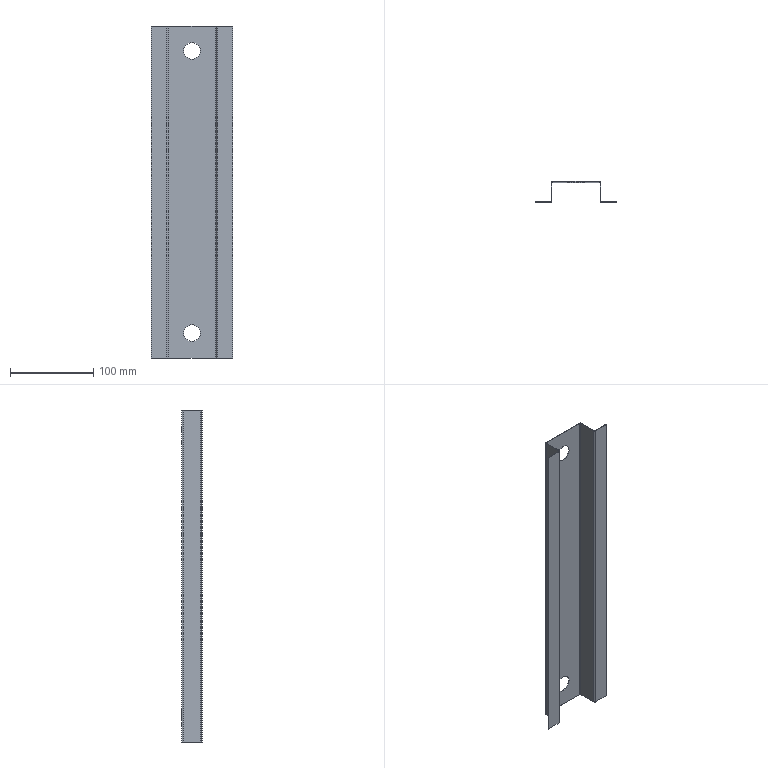Part | 1 solid | 42 faces | box 98.4 x 25 x 400 mm | volume 45704 mm3 | plane 30 | cylinder 12 | commonest cylinder face diameters 2 x4 3.6 x4 20 x4
STEP:
#1=CARTESIAN_POINT('',(10.,-0.8,170.));
#2=VERTEX_POINT('',#1);
#3=CARTESIAN_POINT('',(-10.,-0.8,170.));
#4=VERTEX_POINT('',#3);
#5=CARTESIAN_POINT('',(0.,-0.8,170.));
#6=DIRECTION('',(0.,1.,0.));
#7=DIRECTION('',(-1.,0.,0.));
#8=AXIS2_PLACEMENT_3D('',#5,#6,#7);
#9=CIRCLE('',#8,10.);
#10=EDGE_CURVE('',#2,#4,#9,.T.);
#11=ORIENTED_EDGE('',*,*,#10,.F.);
#12=CARTESIAN_POINT('',(10.,0.,170.));
#13=VERTEX_POINT('',#12);
#14=CARTESIAN_POINT('',(10.,-10.,170.));
#15=DIRECTION('',(0.,1.,0.));
#16=VECTOR('',#15,1000.);
#17=LINE('',#14,#16);
#18=EDGE_CURVE('',#2,#13,#17,.T.);
#19=ORIENTED_EDGE('',*,*,#18,.T.);
#20=CARTESIAN_POINT('',(-10.,0.,170.));
#21=VERTEX_POINT('',#20);
#22=CARTESIAN_POINT('',(0.,0.,170.));
#23=DIRECTION('',(0.,1.,0.));
#24=DIRECTION('',(-1.,0.,0.));
#25=AXIS2_PLACEMENT_3D('',#22,#23,#24);
#26=CIRCLE('',#25,10.);
#27=EDGE_CURVE('',#13,#21,#26,.T.);
#28=ORIENTED_EDGE('',*,*,#27,.T.);
#29=CARTESIAN_POINT('',(-10.,-10.,170.));
#30=DIRECTION('',(0.,1.,0.));
#31=VECTOR('',#30,1000.);
#32=LINE('',#29,#31);
#33=EDGE_CURVE('',#4,#21,#32,.T.);
#34=ORIENTED_EDGE('',*,*,#33,.F.);
#35=EDGE_LOOP('',(#11,#19,#28,#34));
#36=FACE_OUTER_BOUND('',#35,.T.);
#37=CARTESIAN_POINT('',(0.,-10.,170.));
#38=DIRECTION('',(0.,1.,0.));
#39=DIRECTION('',(-1.,0.,0.));
#40=AXIS2_PLACEMENT_3D('',#37,#38,#39);
#41=CYLINDRICAL_SURFACE('',#40,10.);
#42=ADVANCED_FACE('',(#36),#41,.F.);
#43=CARTESIAN_POINT('',(10.,-0.8,-170.));
#44=VERTEX_POINT('',#43);
#45=CARTESIAN_POINT('',(-10.,-0.8,-170.));
#46=VERTEX_POINT('',#45);
#47=CARTESIAN_POINT('',(0.,-0.8,-170.));
#48=DIRECTION('',(0.,1.,0.));
#49=DIRECTION('',(-1.,0.,0.));
#50=AXIS2_PLACEMENT_3D('',#47,#48,#49);
#51=CIRCLE('',#50,10.);
#52=EDGE_CURVE('',#44,#46,#51,.T.);
#53=ORIENTED_EDGE('',*,*,#52,.F.);
#54=CARTESIAN_POINT('',(10.,0.,-170.));
#55=VERTEX_POINT('',#54);
#56=CARTESIAN_POINT('',(10.,-10.,-170.));
#57=DIRECTION('',(0.,1.,0.));
#58=VECTOR('',#57,1000.);
#59=LINE('',#56,#58);
#60=EDGE_CURVE('',#44,#55,#59,.T.);
#61=ORIENTED_EDGE('',*,*,#60,.T.);
#62=CARTESIAN_POINT('',(-10.,0.,-170.));
#63=VERTEX_POINT('',#62);
#64=CARTESIAN_POINT('',(0.,0.,-170.));
#65=DIRECTION('',(0.,1.,0.));
#66=DIRECTION('',(1.,0.,0.));
#67=AXIS2_PLACEMENT_3D('',#64,#65,#66);
#68=CIRCLE('',#67,10.);
#69=EDGE_CURVE('',#55,#63,#68,.T.);
#70=ORIENTED_EDGE('',*,*,#69,.T.);
#71=CARTESIAN_POINT('',(-10.,-10.,-170.));
#72=DIRECTION('',(0.,1.,0.));
#73=VECTOR('',#72,1000.);
#74=LINE('',#71,#73);
#75=EDGE_CURVE('',#46,#63,#74,.T.);
#76=ORIENTED_EDGE('',*,*,#75,.F.);
#77=EDGE_LOOP('',(#53,#61,#70,#76));
#78=FACE_OUTER_BOUND('',#77,.T.);
#79=CARTESIAN_POINT('',(0.,-10.,-170.));
#80=DIRECTION('',(0.,1.,0.));
#81=DIRECTION('',(-1.,0.,0.));
#82=AXIS2_PLACEMENT_3D('',#79,#80,#81);
#83=CYLINDRICAL_SURFACE('',#82,10.);
#84=ADVANCED_FACE('',(#78),#83,.F.);
#85=CARTESIAN_POINT('',(29.2,-23.2,-200.));
#86=VERTEX_POINT('',#85);
#87=CARTESIAN_POINT('',(29.2,-23.2,200.));
#88=VERTEX_POINT('',#87);
#89=CARTESIAN_POINT('',(29.2,-23.2,-200.));
#90=DIRECTION('',(0.,0.,1.));
#91=VECTOR('',#90,1000.);
#92=LINE('',#89,#91);
#93=EDGE_CURVE('',#86,#88,#92,.T.);
#94=ORIENTED_EDGE('',*,*,#93,.T.);
#95=CARTESIAN_POINT('',(29.2,-1.8,200.));
#96=VERTEX_POINT('',#95);
#97=CARTESIAN_POINT('',(29.2,0.,200.));
#98=DIRECTION('',(0.,-1.,0.));
#99=VECTOR('',#98,1000.);
#100=LINE('',#97,#99);
#101=EDGE_CURVE('',#96,#88,#100,.T.);
#102=ORIENTED_EDGE('',*,*,#101,.F.);
#103=CARTESIAN_POINT('',(29.2,-1.8,-200.));
#104=VERTEX_POINT('',#103);
#105=CARTESIAN_POINT('',(29.2,-1.8,200.));
#106=DIRECTION('',(0.,0.,-1.));
#107=VECTOR('',#106,1000.);
#108=LINE('',#105,#107);
#109=EDGE_CURVE('',#96,#104,#108,.T.);
#110=ORIENTED_EDGE('',*,*,#109,.T.);
#111=CARTESIAN_POINT('',(29.2,0.,-200.));
#112=DIRECTION('',(0.,-1.,0.));
#113=VECTOR('',#112,1000.);
#114=LINE('',#111,#113);
#115=EDGE_CURVE('',#104,#86,#114,.T.);
#116=ORIENTED_EDGE('',*,*,#115,.T.);
#117=EDGE_LOOP('',(#94,#102,#110,#116));
#118=FACE_OUTER_BOUND('',#117,.T.);
#119=CARTESIAN_POINT('',(29.2,0.,200.));
#120=DIRECTION('',(1.,0.,0.));
#121=DIRECTION('',(0.,1.,0.));
#122=AXIS2_PLACEMENT_3D('',#119,#120,#121);
#123=PLANE('',#122);
#124=ADVANCED_FACE('',(#118),#123,.F.);
#125=CARTESIAN_POINT('',(30.,-1.8,200.));
#126=VERTEX_POINT('',#125);
#127=CARTESIAN_POINT('',(30.,-23.2,200.));
#128=VERTEX_POINT('',#127);
#129=CARTESIAN_POINT('',(30.,0.,200.));
#130=DIRECTION('',(0.,-1.,0.));
#131=VECTOR('',#130,1000.);
#132=LINE('',#129,#131);
#133=EDGE_CURVE('',#126,#128,#132,.T.);
#134=ORIENTED_EDGE('',*,*,#133,.T.);
#135=CARTESIAN_POINT('',(30.,-23.2,-200.));
#136=VERTEX_POINT('',#135);
#137=CARTESIAN_POINT('',(30.,-23.2,-200.));
#138=DIRECTION('',(0.,0.,1.));
#139=VECTOR('',#138,1000.);
#140=LINE('',#137,#139);
#141=EDGE_CURVE('',#136,#128,#140,.T.);
#142=ORIENTED_EDGE('',*,*,#141,.F.);
#143=CARTESIAN_POINT('',(30.,-1.8,-200.));
#144=VERTEX_POINT('',#143);
#145=CARTESIAN_POINT('',(30.,0.,-200.));
#146=DIRECTION('',(0.,-1.,0.));
#147=VECTOR('',#146,1000.);
#148=LINE('',#145,#147);
#149=EDGE_CURVE('',#144,#136,#148,.T.);
#150=ORIENTED_EDGE('',*,*,#149,.F.);
#151=CARTESIAN_POINT('',(30.,-1.8,200.));
#152=DIRECTION('',(0.,0.,-1.));
#153=VECTOR('',#152,1000.);
#154=LINE('',#151,#153);
#155=EDGE_CURVE('',#126,#144,#154,.T.);
#156=ORIENTED_EDGE('',*,*,#155,.F.);
#157=EDGE_LOOP('',(#134,#142,#150,#156));
#158=FACE_OUTER_BOUND('',#157,.T.);
#159=CARTESIAN_POINT('',(30.,0.,200.));
#160=DIRECTION('',(1.,0.,0.));
#161=DIRECTION('',(0.,1.,0.));
#162=AXIS2_PLACEMENT_3D('',#159,#160,#161);
#163=PLANE('',#162);
#164=ADVANCED_FACE('',(#158),#163,.T.);
#165=CARTESIAN_POINT('',(30.,-23.2,-200.));
#166=DIRECTION('',(-1.,0.,0.));
#167=VECTOR('',#166,1000.);
#168=LINE('',#165,#167);
#169=EDGE_CURVE('',#136,#86,#168,.T.);
#170=ORIENTED_EDGE('',*,*,#169,.T.);
#171=ORIENTED_EDGE('',*,*,#115,.F.);
#172=CARTESIAN_POINT('',(29.2,-1.8,-200.));
#173=DIRECTION('',(1.,0.,0.));
#174=VECTOR('',#173,1000.);
#175=LINE('',#172,#174);
#176=EDGE_CURVE('',#104,#144,#175,.T.);
#177=ORIENTED_EDGE('',*,*,#176,.T.);
#178=ORIENTED_EDGE('',*,*,#149,.T.);
#179=EDGE_LOOP('',(#170,#171,#177,#178));
#180=FACE_OUTER_BOUND('',#179,.T.);
#181=CARTESIAN_POINT('',(28.2,-1.8,-200.));
#182=DIRECTION('',(0.,0.,1.));
#183=DIRECTION('',(1.,0.,0.));
#184=AXIS2_PLACEMENT_3D('',#181,#182,#183);
#185=PLANE('',#184);
#186=ADVANCED_FACE('',(#180),#185,.F.);
#187=CARTESIAN_POINT('',(-30.,-23.2,-200.));
#188=VERTEX_POINT('',#187);
#189=CARTESIAN_POINT('',(-30.,-1.8,-200.));
#190=VERTEX_POINT('',#189);
#191=CARTESIAN_POINT('',(-30.,-25.,-200.));
#192=DIRECTION('',(0.,1.,0.));
#193=VECTOR('',#192,1000.);
#194=LINE('',#191,#193);
#195=EDGE_CURVE('',#188,#190,#194,.T.);
#196=ORIENTED_EDGE('',*,*,#195,.F.);
#197=CARTESIAN_POINT('',(-30.,-23.2,200.));
#198=VERTEX_POINT('',#197);
#199=CARTESIAN_POINT('',(-30.,-23.2,200.));
#200=DIRECTION('',(0.,0.,-1.));
#201=VECTOR('',#200,1000.);
#202=LINE('',#199,#201);
#203=EDGE_CURVE('',#198,#188,#202,.T.);
#204=ORIENTED_EDGE('',*,*,#203,.F.);
#205=CARTESIAN_POINT('',(-30.,-1.8,200.));
#206=VERTEX_POINT('',#205);
#207=CARTESIAN_POINT('',(-30.,-25.,200.));
#208=DIRECTION('',(0.,1.,0.));
#209=VECTOR('',#208,1000.);
#210=LINE('',#207,#209);
#211=EDGE_CURVE('',#198,#206,#210,.T.);
#212=ORIENTED_EDGE('',*,*,#211,.T.);
#213=CARTESIAN_POINT('',(-30.,-1.8,200.));
#214=DIRECTION('',(0.,0.,-1.));
#215=VECTOR('',#214,1000.);
#216=LINE('',#213,#215);
#217=EDGE_CURVE('',#206,#190,#216,.T.);
#218=ORIENTED_EDGE('',*,*,#217,.T.);
#219=EDGE_LOOP('',(#196,#204,#212,#218));
#220=FACE_OUTER_BOUND('',#219,.T.);
#221=CARTESIAN_POINT('',(-30.,-25.,200.));
#222=DIRECTION('',(-1.,0.,0.));
#223=DIRECTION('',(0.,0.,1.));
#224=AXIS2_PLACEMENT_3D('',#221,#222,#223);
#225=PLANE('',#224);
#226=ADVANCED_FACE('',(#220),#225,.T.);
#227=CARTESIAN_POINT('',(-29.2,-23.2,200.));
#228=VERTEX_POINT('',#227);
#229=CARTESIAN_POINT('',(-29.2,-23.2,-200.));
#230=VERTEX_POINT('',#229);
#231=CARTESIAN_POINT('',(-29.2,-23.2,200.));
#232=DIRECTION('',(0.,0.,-1.));
#233=VECTOR('',#232,1000.);
#234=LINE('',#231,#233);
#235=EDGE_CURVE('',#228,#230,#234,.T.);
#236=ORIENTED_EDGE('',*,*,#235,.T.);
#237=CARTESIAN_POINT('',(-29.2,-1.8,-200.));
#238=VERTEX_POINT('',#237);
#239=CARTESIAN_POINT('',(-29.2,-25.,-200.));
#240=DIRECTION('',(0.,1.,0.));
#241=VECTOR('',#240,1000.);
#242=LINE('',#239,#241);
#243=EDGE_CURVE('',#230,#238,#242,.T.);
#244=ORIENTED_EDGE('',*,*,#243,.T.);
#245=CARTESIAN_POINT('',(-29.2,-1.8,200.));
#246=VERTEX_POINT('',#245);
#247=CARTESIAN_POINT('',(-29.2,-1.8,200.));
#248=DIRECTION('',(0.,0.,-1.));
#249=VECTOR('',#248,1000.);
#250=LINE('',#247,#249);
#251=EDGE_CURVE('',#246,#238,#250,.T.);
#252=ORIENTED_EDGE('',*,*,#251,.F.);
#253=CARTESIAN_POINT('',(-29.2,-25.,200.));
#254=DIRECTION('',(0.,1.,0.));
#255=VECTOR('',#254,1000.);
#256=LINE('',#253,#255);
#257=EDGE_CURVE('',#228,#246,#256,.T.);
#258=ORIENTED_EDGE('',*,*,#257,.F.);
#259=EDGE_LOOP('',(#236,#244,#252,#258));
#260=FACE_OUTER_BOUND('',#259,.T.);
#261=CARTESIAN_POINT('',(-29.2,-25.,200.));
#262=DIRECTION('',(-1.,0.,0.));
#263=DIRECTION('',(0.,0.,1.));
#264=AXIS2_PLACEMENT_3D('',#261,#262,#263);
#265=PLANE('',#264);
#266=ADVANCED_FACE('',(#260),#265,.F.);
#267=ORIENTED_EDGE('',*,*,#211,.F.);
#268=CARTESIAN_POINT('',(-30.,-23.2,200.));
#269=DIRECTION('',(1.,0.,0.));
#270=VECTOR('',#269,1000.);
#271=LINE('',#268,#270);
#272=EDGE_CURVE('',#198,#228,#271,.T.);
#273=ORIENTED_EDGE('',*,*,#272,.T.);
#274=ORIENTED_EDGE('',*,*,#257,.T.);
#275=CARTESIAN_POINT('',(-29.2,-1.8,200.));
#276=DIRECTION('',(-1.,0.,0.));
#277=VECTOR('',#276,1000.);
#278=LINE('',#275,#277);
#279=EDGE_CURVE('',#246,#206,#278,.T.);
#280=ORIENTED_EDGE('',*,*,#279,.T.);
#281=EDGE_LOOP('',(#267,#273,#274,#280));
#282=FACE_OUTER_BOUND('',#281,.T.);
#283=CARTESIAN_POINT('',(28.2,-1.8,200.));
#284=DIRECTION('',(0.,0.,1.));
#285=DIRECTION('',(1.,0.,0.));
#286=AXIS2_PLACEMENT_3D('',#283,#284,#285);
#287=PLANE('',#286);
#288=ADVANCED_FACE('',(#282),#287,.T.);
#289=CARTESIAN_POINT('',(-28.2,0.,200.));
#290=VERTEX_POINT('',#289);
#291=CARTESIAN_POINT('',(-28.2,-0.8,200.));
#292=VERTEX_POINT('',#291);
#293=CARTESIAN_POINT('',(-28.2,0.,200.));
#294=DIRECTION('',(0.,-1.,0.));
#295=VECTOR('',#294,1000.);
#296=LINE('',#293,#295);
#297=EDGE_CURVE('',#290,#292,#296,.T.);
#298=ORIENTED_EDGE('',*,*,#297,.F.);
#299=CARTESIAN_POINT('',(-28.2,-1.8,200.));
#300=DIRECTION('',(0.,0.,-1.));
#301=DIRECTION('',(1.,0.,0.));
#302=AXIS2_PLACEMENT_3D('',#299,#300,#301);
#303=CIRCLE('',#302,1.8);
#304=EDGE_CURVE('',#206,#290,#303,.T.);
#305=ORIENTED_EDGE('',*,*,#304,.F.);
#306=ORIENTED_EDGE('',*,*,#279,.F.);
#307=CARTESIAN_POINT('',(-28.2,-1.8,200.));
#308=DIRECTION('',(0.,0.,-1.));
#309=DIRECTION('',(1.,0.,0.));
#310=AXIS2_PLACEMENT_3D('',#307,#308,#309);
#311=CIRCLE('',#310,1.);
#312=EDGE_CURVE('',#246,#292,#311,.T.);
#313=ORIENTED_EDGE('',*,*,#312,.T.);
#314=EDGE_LOOP('',(#298,#305,#306,#313));
#315=FACE_OUTER_BOUND('',#314,.T.);
#316=CARTESIAN_POINT('',(-28.2,0.,200.));
#317=DIRECTION('',(0.,0.,1.));
#318=DIRECTION('',(1.,0.,0.));
#319=AXIS2_PLACEMENT_3D('',#316,#317,#318);
#320=PLANE('',#319);
#321=ADVANCED_FACE('',(#315),#320,.T.);
#322=CARTESIAN_POINT('',(28.2,0.,200.));
#323=VERTEX_POINT('',#322);
#324=CARTESIAN_POINT('',(-30.,0.,200.));
#325=DIRECTION('',(1.,0.,0.));
#326=VECTOR('',#325,1000.);
#327=LINE('',#324,#326);
#328=EDGE_CURVE('',#290,#323,#327,.T.);
#329=ORIENTED_EDGE('',*,*,#328,.F.);
#330=ORIENTED_EDGE('',*,*,#297,.T.);
#331=CARTESIAN_POINT('',(28.2,-0.8,200.));
#332=VERTEX_POINT('',#331);
#333=CARTESIAN_POINT('',(-30.,-0.8,200.));
#334=DIRECTION('',(1.,0.,0.));
#335=VECTOR('',#334,1000.);
#336=LINE('',#333,#335);
#337=EDGE_CURVE('',#292,#332,#336,.T.);
#338=ORIENTED_EDGE('',*,*,#337,.T.);
#339=CARTESIAN_POINT('',(28.2,-0.8,200.));
#340=DIRECTION('',(0.,1.,0.));
#341=VECTOR('',#340,1000.);
#342=LINE('',#339,#341);
#343=EDGE_CURVE('',#332,#323,#342,.T.);
#344=ORIENTED_EDGE('',*,*,#343,.T.);
#345=EDGE_LOOP('',(#329,#330,#338,#344));
#346=FACE_OUTER_BOUND('',#345,.T.);
#347=CARTESIAN_POINT('',(-29.2,-1.8,200.));
#348=DIRECTION('',(0.,0.,1.));
#349=DIRECTION('',(1.,0.,0.));
#350=AXIS2_PLACEMENT_3D('',#347,#348,#349);
#351=PLANE('',#350);
#352=ADVANCED_FACE('',(#346),#351,.T.);
#353=CARTESIAN_POINT('',(-30.,-1.8,-200.));
#354=DIRECTION('',(1.,0.,0.));
#355=VECTOR('',#354,1000.);
#356=LINE('',#353,#355);
#357=EDGE_CURVE('',#190,#238,#356,.T.);
#358=ORIENTED_EDGE('',*,*,#357,.F.);
#359=CARTESIAN_POINT('',(-28.2,0.,-200.));
#360=VERTEX_POINT('',#359);
#361=CARTESIAN_POINT('',(-28.2,-1.8,-200.));
#362=DIRECTION('',(0.,0.,-1.));
#363=DIRECTION('',(1.,0.,0.));
#364=AXIS2_PLACEMENT_3D('',#361,#362,#363);
#365=CIRCLE('',#364,1.8);
#366=EDGE_CURVE('',#190,#360,#365,.T.);
#367=ORIENTED_EDGE('',*,*,#366,.T.);
#368=CARTESIAN_POINT('',(-28.2,-0.8,-200.));
#369=VERTEX_POINT('',#368);
#370=CARTESIAN_POINT('',(-28.2,-0.8,-200.));
#371=DIRECTION('',(0.,1.,0.));
#372=VECTOR('',#371,1000.);
#373=LINE('',#370,#372);
#374=EDGE_CURVE('',#369,#360,#373,.T.);
#375=ORIENTED_EDGE('',*,*,#374,.F.);
#376=CARTESIAN_POINT('',(-28.2,-1.8,-200.));
#377=DIRECTION('',(0.,0.,-1.));
#378=DIRECTION('',(1.,0.,0.));
#379=AXIS2_PLACEMENT_3D('',#376,#377,#378);
#380=CIRCLE('',#379,1.);
#381=EDGE_CURVE('',#238,#369,#380,.T.);
#382=ORIENTED_EDGE('',*,*,#381,.F.);
#383=EDGE_LOOP('',(#358,#367,#375,#382));
#384=FACE_OUTER_BOUND('',#383,.T.);
#385=CARTESIAN_POINT('',(-30.,-1.8,-200.));
#386=DIRECTION('',(0.,0.,-1.));
#387=DIRECTION('',(-1.,0.,0.));
#388=AXIS2_PLACEMENT_3D('',#385,#386,#387);
#389=PLANE('',#388);
#390=ADVANCED_FACE('',(#384),#389,.T.);
#391=CARTESIAN_POINT('',(-30.,-23.2,-200.));
#392=DIRECTION('',(1.,0.,0.));
#393=VECTOR('',#392,1000.);
#394=LINE('',#391,#393);
#395=EDGE_CURVE('',#188,#230,#394,.T.);
#396=ORIENTED_EDGE('',*,*,#395,.F.);
#397=ORIENTED_EDGE('',*,*,#195,.T.);
#398=ORIENTED_EDGE('',*,*,#357,.T.);
#399=ORIENTED_EDGE('',*,*,#243,.F.);
#400=EDGE_LOOP('',(#396,#397,#398,#399));
#401=FACE_OUTER_BOUND('',#400,.T.);
#402=CARTESIAN_POINT('',(-28.2,-0.8,-200.));
#403=DIRECTION('',(0.,0.,-1.));
#404=DIRECTION('',(-1.,0.,0.));
#405=AXIS2_PLACEMENT_3D('',#402,#403,#404);
#406=PLANE('',#405);
#407=ADVANCED_FACE('',(#401),#406,.T.);
#408=CARTESIAN_POINT('',(30.,-1.8,200.));
#409=DIRECTION('',(-1.,0.,0.));
#410=VECTOR('',#409,1000.);
#411=LINE('',#408,#410);
#412=EDGE_CURVE('',#126,#96,#411,.T.);
#413=ORIENTED_EDGE('',*,*,#412,.F.);
#414=CARTESIAN_POINT('',(28.2,-1.8,200.));
#415=DIRECTION('',(0.,0.,-1.));
#416=DIRECTION('',(1.,0.,0.));
#417=AXIS2_PLACEMENT_3D('',#414,#415,#416);
#418=CIRCLE('',#417,1.8);
#419=EDGE_CURVE('',#323,#126,#418,.T.);
#420=ORIENTED_EDGE('',*,*,#419,.F.);
#421=ORIENTED_EDGE('',*,*,#343,.F.);
#422=CARTESIAN_POINT('',(28.2,-1.8,200.));
#423=DIRECTION('',(0.,0.,-1.));
#424=DIRECTION('',(1.,0.,0.));
#425=AXIS2_PLACEMENT_3D('',#422,#423,#424);
#426=CIRCLE('',#425,1.);
#427=EDGE_CURVE('',#332,#96,#426,.T.);
#428=ORIENTED_EDGE('',*,*,#427,.T.);
#429=EDGE_LOOP('',(#413,#420,#421,#428));
#430=FACE_OUTER_BOUND('',#429,.T.);
#431=CARTESIAN_POINT('',(30.,-1.8,200.));
#432=DIRECTION('',(0.,0.,1.));
#433=DIRECTION('',(1.,0.,0.));
#434=AXIS2_PLACEMENT_3D('',#431,#432,#433);
#435=PLANE('',#434);
#436=ADVANCED_FACE('',(#430),#435,.T.);
#437=CARTESIAN_POINT('',(30.,-23.2,200.));
#438=DIRECTION('',(-1.,0.,0.));
#439=VECTOR('',#438,1000.);
#440=LINE('',#437,#439);
#441=EDGE_CURVE('',#128,#88,#440,.T.);
#442=ORIENTED_EDGE('',*,*,#441,.F.);
#443=ORIENTED_EDGE('',*,*,#133,.F.);
#444=ORIENTED_EDGE('',*,*,#412,.T.);
#445=ORIENTED_EDGE('',*,*,#101,.T.);
#446=EDGE_LOOP('',(#442,#443,#444,#445));
#447=FACE_OUTER_BOUND('',#446,.T.);
#448=CARTESIAN_POINT('',(28.2,-0.8,200.));
#449=DIRECTION('',(0.,0.,1.));
#450=DIRECTION('',(1.,0.,0.));
#451=AXIS2_PLACEMENT_3D('',#448,#449,#450);
#452=PLANE('',#451);
#453=ADVANCED_FACE('',(#447),#452,.T.);
#454=CARTESIAN_POINT('',(28.2,0.,-200.));
#455=VERTEX_POINT('',#454);
#456=CARTESIAN_POINT('',(28.2,-0.8,-200.));
#457=VERTEX_POINT('',#456);
#458=CARTESIAN_POINT('',(28.2,0.,-200.));
#459=DIRECTION('',(0.,-1.,0.));
#460=VECTOR('',#459,1000.);
#461=LINE('',#458,#460);
#462=EDGE_CURVE('',#455,#457,#461,.T.);
#463=ORIENTED_EDGE('',*,*,#462,.F.);
#464=CARTESIAN_POINT('',(28.2,-1.8,-200.));
#465=DIRECTION('',(0.,0.,-1.));
#466=DIRECTION('',(1.,0.,0.));
#467=AXIS2_PLACEMENT_3D('',#464,#465,#466);
#468=CIRCLE('',#467,1.8);
#469=EDGE_CURVE('',#455,#144,#468,.T.);
#470=ORIENTED_EDGE('',*,*,#469,.T.);
#471=ORIENTED_EDGE('',*,*,#176,.F.);
#472=CARTESIAN_POINT('',(28.2,-1.8,-200.));
#473=DIRECTION('',(0.,0.,-1.));
#474=DIRECTION('',(1.,0.,0.));
#475=AXIS2_PLACEMENT_3D('',#472,#473,#474);
#476=CIRCLE('',#475,1.);
#477=EDGE_CURVE('',#457,#104,#476,.T.);
#478=ORIENTED_EDGE('',*,*,#477,.F.);
#479=EDGE_LOOP('',(#463,#470,#471,#478));
#480=FACE_OUTER_BOUND('',#479,.T.);
#481=CARTESIAN_POINT('',(28.2,0.,-200.));
#482=DIRECTION('',(0.,0.,-1.));
#483=DIRECTION('',(-1.,0.,0.));
#484=AXIS2_PLACEMENT_3D('',#481,#482,#483);
#485=PLANE('',#484);
#486=ADVANCED_FACE('',(#480),#485,.T.);
#487=CARTESIAN_POINT('',(-30.,0.,-200.));
#488=DIRECTION('',(1.,0.,0.));
#489=VECTOR('',#488,1000.);
#490=LINE('',#487,#489);
#491=EDGE_CURVE('',#360,#455,#490,.T.);
#492=ORIENTED_EDGE('',*,*,#491,.T.);
#493=ORIENTED_EDGE('',*,*,#462,.T.);
#494=CARTESIAN_POINT('',(-30.,-0.8,-200.));
#495=DIRECTION('',(1.,0.,0.));
#496=VECTOR('',#495,1000.);
#497=LINE('',#494,#496);
#498=EDGE_CURVE('',#369,#457,#497,.T.);
#499=ORIENTED_EDGE('',*,*,#498,.F.);
#500=ORIENTED_EDGE('',*,*,#374,.T.);
#501=EDGE_LOOP('',(#492,#493,#499,#500));
#502=FACE_OUTER_BOUND('',#501,.T.);
#503=CARTESIAN_POINT('',(29.2,-1.8,-200.));
#504=DIRECTION('',(0.,0.,-1.));
#505=DIRECTION('',(-1.,0.,0.));
#506=AXIS2_PLACEMENT_3D('',#503,#504,#505);
#507=PLANE('',#506);
#508=ADVANCED_FACE('',(#502),#507,.T.);
#509=ORIENTED_EDGE('',*,*,#469,.F.);
#510=CARTESIAN_POINT('',(28.2,0.,200.));
#511=DIRECTION('',(0.,0.,-1.));
#512=VECTOR('',#511,1000.);
#513=LINE('',#510,#512);
#514=EDGE_CURVE('',#323,#455,#513,.T.);
#515=ORIENTED_EDGE('',*,*,#514,.F.);
#516=ORIENTED_EDGE('',*,*,#419,.T.);
#517=ORIENTED_EDGE('',*,*,#155,.T.);
#518=EDGE_LOOP('',(#509,#515,#516,#517));
#519=FACE_OUTER_BOUND('',#518,.T.);
#520=CARTESIAN_POINT('',(28.2,-1.8,200.));
#521=DIRECTION('',(0.,0.,-1.));
#522=DIRECTION('',(-1.,0.,0.));
#523=AXIS2_PLACEMENT_3D('',#520,#521,#522);
#524=CYLINDRICAL_SURFACE('',#523,1.8);
#525=ADVANCED_FACE('',(#519),#524,.T.);
#526=CARTESIAN_POINT('',(0.,0.,170.));
#527=DIRECTION('',(0.,1.,0.));
#528=DIRECTION('',(-1.,0.,0.));
#529=AXIS2_PLACEMENT_3D('',#526,#527,#528);
#530=CIRCLE('',#529,10.);
#531=EDGE_CURVE('',#21,#13,#530,.T.);
#532=ORIENTED_EDGE('',*,*,#531,.F.);
#533=ORIENTED_EDGE('',*,*,#27,.F.);
#534=EDGE_LOOP('',(#532,#533));
#535=FACE_BOUND('',#534,.T.);
#536=CARTESIAN_POINT('',(0.,0.,-170.));
#537=DIRECTION('',(0.,1.,0.));
#538=DIRECTION('',(1.,0.,0.));
#539=AXIS2_PLACEMENT_3D('',#536,#537,#538);
#540=CIRCLE('',#539,10.);
#541=EDGE_CURVE('',#63,#55,#540,.T.);
#542=ORIENTED_EDGE('',*,*,#541,.F.);
#543=ORIENTED_EDGE('',*,*,#69,.F.);
#544=EDGE_LOOP('',(#542,#543));
#545=FACE_BOUND('',#544,.T.);
#546=ORIENTED_EDGE('',*,*,#491,.F.);
#547=CARTESIAN_POINT('',(-28.2,0.,200.));
#548=DIRECTION('',(0.,0.,-1.));
#549=VECTOR('',#548,1000.);
#550=LINE('',#547,#549);
#551=EDGE_CURVE('',#290,#360,#550,.T.);
#552=ORIENTED_EDGE('',*,*,#551,.F.);
#553=ORIENTED_EDGE('',*,*,#328,.T.);
#554=ORIENTED_EDGE('',*,*,#514,.T.);
#555=EDGE_LOOP('',(#546,#552,#553,#554));
#556=FACE_OUTER_BOUND('',#555,.T.);
#557=CARTESIAN_POINT('',(-30.,0.,200.));
#558=DIRECTION('',(0.,1.,0.));
#559=DIRECTION('',(-1.,0.,0.));
#560=AXIS2_PLACEMENT_3D('',#557,#558,#559);
#561=PLANE('',#560);
#562=ADVANCED_FACE('',(#535,#545,#556),#561,.T.);
#563=ORIENTED_EDGE('',*,*,#366,.F.);
#564=ORIENTED_EDGE('',*,*,#217,.F.);
#565=ORIENTED_EDGE('',*,*,#304,.T.);
#566=ORIENTED_EDGE('',*,*,#551,.T.);
#567=EDGE_LOOP('',(#563,#564,#565,#566));
#568=FACE_OUTER_BOUND('',#567,.T.);
#569=CARTESIAN_POINT('',(-28.2,-1.8,200.));
#570=DIRECTION('',(0.,0.,-1.));
#571=DIRECTION('',(-1.,0.,0.));
#572=AXIS2_PLACEMENT_3D('',#569,#570,#571);
#573=CYLINDRICAL_SURFACE('',#572,1.8);
#574=ADVANCED_FACE('',(#568),#573,.T.);
#575=ORIENTED_EDGE('',*,*,#381,.T.);
#576=CARTESIAN_POINT('',(-28.2,-0.8,200.));
#577=DIRECTION('',(0.,0.,-1.));
#578=VECTOR('',#577,1000.);
#579=LINE('',#576,#578);
#580=EDGE_CURVE('',#292,#369,#579,.T.);
#581=ORIENTED_EDGE('',*,*,#580,.F.);
#582=ORIENTED_EDGE('',*,*,#312,.F.);
#583=ORIENTED_EDGE('',*,*,#251,.T.);
#584=EDGE_LOOP('',(#575,#581,#582,#583));
#585=FACE_OUTER_BOUND('',#584,.T.);
#586=CARTESIAN_POINT('',(-28.2,-1.8,200.));
#587=DIRECTION('',(0.,0.,-1.));
#588=DIRECTION('',(-1.,0.,0.));
#589=AXIS2_PLACEMENT_3D('',#586,#587,#588);
#590=CYLINDRICAL_SURFACE('',#589,1.);
#591=ADVANCED_FACE('',(#585),#590,.F.);
#592=CARTESIAN_POINT('',(0.,-0.8,170.));
#593=DIRECTION('',(0.,1.,0.));
#594=DIRECTION('',(-1.,0.,0.));
#595=AXIS2_PLACEMENT_3D('',#592,#593,#594);
#596=CIRCLE('',#595,10.);
#597=EDGE_CURVE('',#4,#2,#596,.T.);
#598=ORIENTED_EDGE('',*,*,#597,.T.);
#599=ORIENTED_EDGE('',*,*,#10,.T.);
#600=EDGE_LOOP('',(#598,#599));
#601=FACE_BOUND('',#600,.T.);
#602=CARTESIAN_POINT('',(0.,-0.8,-170.));
#603=DIRECTION('',(0.,1.,0.));
#604=DIRECTION('',(-1.,0.,0.));
#605=AXIS2_PLACEMENT_3D('',#602,#603,#604);
#606=CIRCLE('',#605,10.);
#607=EDGE_CURVE('',#46,#44,#606,.T.);
#608=ORIENTED_EDGE('',*,*,#607,.T.);
#609=ORIENTED_EDGE('',*,*,#52,.T.);
#610=EDGE_LOOP('',(#608,#609));
#611=FACE_BOUND('',#610,.T.);
#612=ORIENTED_EDGE('',*,*,#498,.T.);
#613=CARTESIAN_POINT('',(28.2,-0.8,200.));
#614=DIRECTION('',(0.,0.,-1.));
#615=VECTOR('',#614,1000.);
#616=LINE('',#613,#615);
#617=EDGE_CURVE('',#332,#457,#616,.T.);
#618=ORIENTED_EDGE('',*,*,#617,.F.);
#619=ORIENTED_EDGE('',*,*,#337,.F.);
#620=ORIENTED_EDGE('',*,*,#580,.T.);
#621=EDGE_LOOP('',(#612,#618,#619,#620));
#622=FACE_OUTER_BOUND('',#621,.T.);
#623=CARTESIAN_POINT('',(-30.,-0.8,200.));
#624=DIRECTION('',(0.,1.,0.));
#625=DIRECTION('',(-1.,0.,0.));
#626=AXIS2_PLACEMENT_3D('',#623,#624,#625);
#627=PLANE('',#626);
#628=ADVANCED_FACE('',(#601,#611,#622),#627,.F.);
#629=ORIENTED_EDGE('',*,*,#477,.T.);
#630=ORIENTED_EDGE('',*,*,#109,.F.);
#631=ORIENTED_EDGE('',*,*,#427,.F.);
#632=ORIENTED_EDGE('',*,*,#617,.T.);
#633=EDGE_LOOP('',(#629,#630,#631,#632));
#634=FACE_OUTER_BOUND('',#633,.T.);
#635=CARTESIAN_POINT('',(28.2,-1.8,200.));
#636=DIRECTION('',(0.,0.,-1.));
#637=DIRECTION('',(-1.,0.,0.));
#638=AXIS2_PLACEMENT_3D('',#635,#636,#637);
#639=CYLINDRICAL_SURFACE('',#638,1.);
#640=ADVANCED_FACE('',(#634),#639,.F.);
#641=CARTESIAN_POINT('',(-31.,-24.2,-200.));
#642=VERTEX_POINT('',#641);
#643=CARTESIAN_POINT('',(-31.,-25.,-200.));
#644=VERTEX_POINT('',#643);
#645=CARTESIAN_POINT('',(-31.,-25.,-200.));
#646=DIRECTION('',(0.,-1.,0.));
#647=VECTOR('',#646,1000.);
#648=LINE('',#645,#647);
#649=EDGE_CURVE('',#642,#644,#648,.T.);
#650=ORIENTED_EDGE('',*,*,#649,.F.);
#651=CARTESIAN_POINT('',(-31.,-23.2,-200.));
#652=DIRECTION('',(0.,0.,-1.));
#653=DIRECTION('',(1.,0.,0.));
#654=AXIS2_PLACEMENT_3D('',#651,#652,#653);
#655=CIRCLE('',#654,1.);
#656=EDGE_CURVE('',#188,#642,#655,.T.);
#657=ORIENTED_EDGE('',*,*,#656,.F.);
#658=ORIENTED_EDGE('',*,*,#395,.T.);
#659=CARTESIAN_POINT('',(-31.,-23.2,-200.));
#660=DIRECTION('',(0.,0.,-1.));
#661=DIRECTION('',(1.,0.,0.));
#662=AXIS2_PLACEMENT_3D('',#659,#660,#661);
#663=CIRCLE('',#662,1.8);
#664=EDGE_CURVE('',#230,#644,#663,.T.);
#665=ORIENTED_EDGE('',*,*,#664,.T.);
#666=EDGE_LOOP('',(#650,#657,#658,#665));
#667=FACE_OUTER_BOUND('',#666,.T.);
#668=CARTESIAN_POINT('',(-31.,-23.2,-200.));
#669=DIRECTION('',(0.,0.,-1.));
#670=DIRECTION('',(-1.,0.,0.));
#671=AXIS2_PLACEMENT_3D('',#668,#669,#670);
#672=PLANE('',#671);
#673=ADVANCED_FACE('',(#667),#672,.T.);
#674=CARTESIAN_POINT('',(-31.,-24.2,200.));
#675=VERTEX_POINT('',#674);
#676=CARTESIAN_POINT('',(-31.,-23.2,200.));
#677=DIRECTION('',(0.,0.,1.));
#678=DIRECTION('',(1.,0.,0.));
#679=AXIS2_PLACEMENT_3D('',#676,#677,#678);
#680=CIRCLE('',#679,1.);
#681=EDGE_CURVE('',#675,#198,#680,.T.);
#682=ORIENTED_EDGE('',*,*,#681,.F.);
#683=CARTESIAN_POINT('',(-31.,-25.,200.));
#684=VERTEX_POINT('',#683);
#685=CARTESIAN_POINT('',(-31.,-24.2,200.));
#686=DIRECTION('',(0.,-1.,0.));
#687=VECTOR('',#686,1000.);
#688=LINE('',#685,#687);
#689=EDGE_CURVE('',#675,#684,#688,.T.);
#690=ORIENTED_EDGE('',*,*,#689,.T.);
#691=CARTESIAN_POINT('',(-31.,-23.2,200.));
#692=DIRECTION('',(0.,0.,1.));
#693=DIRECTION('',(1.,0.,0.));
#694=AXIS2_PLACEMENT_3D('',#691,#692,#693);
#695=CIRCLE('',#694,1.8);
#696=EDGE_CURVE('',#684,#228,#695,.T.);
#697=ORIENTED_EDGE('',*,*,#696,.T.);
#698=ORIENTED_EDGE('',*,*,#272,.F.);
#699=EDGE_LOOP('',(#682,#690,#697,#698));
#700=FACE_OUTER_BOUND('',#699,.T.);
#701=CARTESIAN_POINT('',(-31.,-23.2,200.));
#702=DIRECTION('',(0.,0.,-1.));
#703=DIRECTION('',(-1.,0.,0.));
#704=AXIS2_PLACEMENT_3D('',#701,#702,#703);
#705=PLANE('',#704);
#706=ADVANCED_FACE('',(#700),#705,.F.);
#707=ORIENTED_EDGE('',*,*,#235,.F.);
#708=ORIENTED_EDGE('',*,*,#696,.F.);
#709=CARTESIAN_POINT('',(-31.,-25.,-200.));
#710=DIRECTION('',(0.,0.,-1.));
#711=VECTOR('',#710,1000.);
#712=LINE('',#709,#711);
#713=EDGE_CURVE('',#684,#644,#712,.T.);
#714=ORIENTED_EDGE('',*,*,#713,.T.);
#715=ORIENTED_EDGE('',*,*,#664,.F.);
#716=EDGE_LOOP('',(#707,#708,#714,#715));
#717=FACE_OUTER_BOUND('',#716,.T.);
#718=CARTESIAN_POINT('',(-31.,-23.2,200.));
#719=DIRECTION('',(0.,0.,1.));
#720=DIRECTION('',(0.,-1.,0.));
#721=AXIS2_PLACEMENT_3D('',#718,#719,#720);
#722=CYLINDRICAL_SURFACE('',#721,1.8);
#723=ADVANCED_FACE('',(#717),#722,.T.);
#724=ORIENTED_EDGE('',*,*,#203,.T.);
#725=ORIENTED_EDGE('',*,*,#656,.T.);
#726=CARTESIAN_POINT('',(-31.,-24.2,-200.));
#727=DIRECTION('',(0.,0.,1.));
#728=VECTOR('',#727,1000.);
#729=LINE('',#726,#728);
#730=EDGE_CURVE('',#642,#675,#729,.T.);
#731=ORIENTED_EDGE('',*,*,#730,.T.);
#732=ORIENTED_EDGE('',*,*,#681,.T.);
#733=EDGE_LOOP('',(#724,#725,#731,#732));
#734=FACE_OUTER_BOUND('',#733,.T.);
#735=CARTESIAN_POINT('',(-31.,-23.2,200.));
#736=DIRECTION('',(0.,0.,1.));
#737=DIRECTION('',(0.,-1.,0.));
#738=AXIS2_PLACEMENT_3D('',#735,#736,#737);
#739=CYLINDRICAL_SURFACE('',#738,1.);
#740=ADVANCED_FACE('',(#734),#739,.F.);
#741=ORIENTED_EDGE('',*,*,#689,.F.);
#742=CARTESIAN_POINT('',(-49.2,-24.2,200.));
#743=VERTEX_POINT('',#742);
#744=CARTESIAN_POINT('',(-49.2,-24.2,200.));
#745=DIRECTION('',(-1.,0.,0.));
#746=VECTOR('',#745,1000.);
#747=LINE('',#744,#746);
#748=EDGE_CURVE('',#675,#743,#747,.T.);
#749=ORIENTED_EDGE('',*,*,#748,.T.);
#750=CARTESIAN_POINT('',(-49.2,-25.,200.));
#751=VERTEX_POINT('',#750);
#752=CARTESIAN_POINT('',(-49.2,-25.,200.));
#753=DIRECTION('',(0.,1.,0.));
#754=VECTOR('',#753,1000.);
#755=LINE('',#752,#754);
#756=EDGE_CURVE('',#751,#743,#755,.T.);
#757=ORIENTED_EDGE('',*,*,#756,.F.);
#758=CARTESIAN_POINT('',(0.,-25.,200.));
#759=DIRECTION('',(-1.,0.,0.));
#760=VECTOR('',#759,1000.);
#761=LINE('',#758,#760);
#762=EDGE_CURVE('',#684,#751,#761,.T.);
#763=ORIENTED_EDGE('',*,*,#762,.F.);
#764=EDGE_LOOP('',(#741,#749,#757,#763));
#765=FACE_OUTER_BOUND('',#764,.T.);
#766=CARTESIAN_POINT('',(-49.2,-25.,200.));
#767=DIRECTION('',(0.,0.,-1.));
#768=DIRECTION('',(-1.,0.,0.));
#769=AXIS2_PLACEMENT_3D('',#766,#767,#768);
#770=PLANE('',#769);
#771=ADVANCED_FACE('',(#765),#770,.F.);
#772=ORIENTED_EDGE('',*,*,#649,.T.);
#773=CARTESIAN_POINT('',(-49.2,-25.,-200.));
#774=VERTEX_POINT('',#773);
#775=CARTESIAN_POINT('',(0.,-25.,-200.));
#776=DIRECTION('',(1.,0.,0.));
#777=VECTOR('',#776,1000.);
#778=LINE('',#775,#777);
#779=EDGE_CURVE('',#774,#644,#778,.T.);
#780=ORIENTED_EDGE('',*,*,#779,.F.);
#781=CARTESIAN_POINT('',(-49.2,-24.2,-200.));
#782=VERTEX_POINT('',#781);
#783=CARTESIAN_POINT('',(-49.2,-25.,-200.));
#784=DIRECTION('',(0.,1.,0.));
#785=VECTOR('',#784,1000.);
#786=LINE('',#783,#785);
#787=EDGE_CURVE('',#774,#782,#786,.T.);
#788=ORIENTED_EDGE('',*,*,#787,.T.);
#789=CARTESIAN_POINT('',(-30.,-24.2,-200.));
#790=DIRECTION('',(1.,0.,0.));
#791=VECTOR('',#790,1000.);
#792=LINE('',#789,#791);
#793=EDGE_CURVE('',#782,#642,#792,.T.);
#794=ORIENTED_EDGE('',*,*,#793,.T.);
#795=EDGE_LOOP('',(#772,#780,#788,#794));
#796=FACE_OUTER_BOUND('',#795,.T.);
#797=CARTESIAN_POINT('',(-30.,-25.,-200.));
#798=DIRECTION('',(0.,0.,1.));
#799=DIRECTION('',(1.,0.,0.));
#800=AXIS2_PLACEMENT_3D('',#797,#798,#799);
#801=PLANE('',#800);
#802=ADVANCED_FACE('',(#796),#801,.F.);
#803=ORIENTED_EDGE('',*,*,#713,.F.);
#804=ORIENTED_EDGE('',*,*,#762,.T.);
#805=CARTESIAN_POINT('',(-49.2,-25.,0.));
#806=DIRECTION('',(0.,0.,-1.));
#807=VECTOR('',#806,1000.);
#808=LINE('',#805,#807);
#809=EDGE_CURVE('',#751,#774,#808,.T.);
#810=ORIENTED_EDGE('',*,*,#809,.T.);
#811=ORIENTED_EDGE('',*,*,#779,.T.);
#812=EDGE_LOOP('',(#803,#804,#810,#811));
#813=FACE_OUTER_BOUND('',#812,.T.);
#814=CARTESIAN_POINT('',(0.,-25.,0.));
#815=DIRECTION('',(0.,1.,0.));
#816=DIRECTION('',(-1.,0.,0.));
#817=AXIS2_PLACEMENT_3D('',#814,#815,#816);
#818=PLANE('',#817);
#819=ADVANCED_FACE('',(#813),#818,.F.);
#820=ORIENTED_EDGE('',*,*,#748,.F.);
#821=ORIENTED_EDGE('',*,*,#730,.F.);
#822=ORIENTED_EDGE('',*,*,#793,.F.);
#823=CARTESIAN_POINT('',(-49.2,-24.2,-200.));
#824=DIRECTION('',(0.,0.,-1.));
#825=VECTOR('',#824,1000.);
#826=LINE('',#823,#825);
#827=EDGE_CURVE('',#743,#782,#826,.T.);
#828=ORIENTED_EDGE('',*,*,#827,.F.);
#829=EDGE_LOOP('',(#820,#821,#822,#828));
#830=FACE_OUTER_BOUND('',#829,.T.);
#831=CARTESIAN_POINT('',(0.,-24.2,0.));
#832=DIRECTION('',(0.,1.,0.));
#833=DIRECTION('',(-1.,0.,0.));
#834=AXIS2_PLACEMENT_3D('',#831,#832,#833);
#835=PLANE('',#834);
#836=ADVANCED_FACE('',(#830),#835,.T.);
#837=ORIENTED_EDGE('',*,*,#827,.T.);
#838=ORIENTED_EDGE('',*,*,#787,.F.);
#839=ORIENTED_EDGE('',*,*,#809,.F.);
#840=ORIENTED_EDGE('',*,*,#756,.T.);
#841=EDGE_LOOP('',(#837,#838,#839,#840));
#842=FACE_OUTER_BOUND('',#841,.T.);
#843=CARTESIAN_POINT('',(-49.2,-25.,-200.));
#844=DIRECTION('',(1.,0.,0.));
#845=DIRECTION('',(0.,1.,0.));
#846=AXIS2_PLACEMENT_3D('',#843,#844,#845);
#847=PLANE('',#846);
#848=ADVANCED_FACE('',(#842),#847,.F.);
#849=CARTESIAN_POINT('',(31.,-24.2,200.));
#850=VERTEX_POINT('',#849);
#851=CARTESIAN_POINT('',(31.,-25.,200.));
#852=VERTEX_POINT('',#851);
#853=CARTESIAN_POINT('',(31.,-25.,200.));
#854=DIRECTION('',(0.,-1.,0.));
#855=VECTOR('',#854,1000.);
#856=LINE('',#853,#855);
#857=EDGE_CURVE('',#850,#852,#856,.T.);
#858=ORIENTED_EDGE('',*,*,#857,.F.);
#859=CARTESIAN_POINT('',(31.,-23.2,200.));
#860=DIRECTION('',(0.,0.,1.));
#861=DIRECTION('',(-1.,0.,0.));
#862=AXIS2_PLACEMENT_3D('',#859,#860,#861);
#863=CIRCLE('',#862,1.);
#864=EDGE_CURVE('',#128,#850,#863,.T.);
#865=ORIENTED_EDGE('',*,*,#864,.F.);
#866=ORIENTED_EDGE('',*,*,#441,.T.);
#867=CARTESIAN_POINT('',(31.,-23.2,200.));
#868=DIRECTION('',(0.,0.,1.));
#869=DIRECTION('',(-1.,0.,0.));
#870=AXIS2_PLACEMENT_3D('',#867,#868,#869);
#871=CIRCLE('',#870,1.8);
#872=EDGE_CURVE('',#88,#852,#871,.T.);
#873=ORIENTED_EDGE('',*,*,#872,.T.);
#874=EDGE_LOOP('',(#858,#865,#866,#873));
#875=FACE_OUTER_BOUND('',#874,.T.);
#876=CARTESIAN_POINT('',(31.,-23.2,200.));
#877=DIRECTION('',(0.,0.,1.));
#878=DIRECTION('',(1.,0.,0.));
#879=AXIS2_PLACEMENT_3D('',#876,#877,#878);
#880=PLANE('',#879);
#881=ADVANCED_FACE('',(#875),#880,.T.);
#882=CARTESIAN_POINT('',(31.,-24.2,-200.));
#883=VERTEX_POINT('',#882);
#884=CARTESIAN_POINT('',(31.,-23.2,-200.));
#885=DIRECTION('',(0.,0.,-1.));
#886=DIRECTION('',(-1.,0.,0.));
#887=AXIS2_PLACEMENT_3D('',#884,#885,#886);
#888=CIRCLE('',#887,1.);
#889=EDGE_CURVE('',#883,#136,#888,.T.);
#890=ORIENTED_EDGE('',*,*,#889,.F.);
#891=CARTESIAN_POINT('',(31.,-25.,-200.));
#892=VERTEX_POINT('',#891);
#893=CARTESIAN_POINT('',(31.,-24.2,-200.));
#894=DIRECTION('',(0.,-1.,0.));
#895=VECTOR('',#894,1000.);
#896=LINE('',#893,#895);
#897=EDGE_CURVE('',#883,#892,#896,.T.);
#898=ORIENTED_EDGE('',*,*,#897,.T.);
#899=CARTESIAN_POINT('',(31.,-23.2,-200.));
#900=DIRECTION('',(0.,0.,-1.));
#901=DIRECTION('',(-1.,0.,0.));
#902=AXIS2_PLACEMENT_3D('',#899,#900,#901);
#903=CIRCLE('',#902,1.8);
#904=EDGE_CURVE('',#892,#86,#903,.T.);
#905=ORIENTED_EDGE('',*,*,#904,.T.);
#906=ORIENTED_EDGE('',*,*,#169,.F.);
#907=EDGE_LOOP('',(#890,#898,#905,#906));
#908=FACE_OUTER_BOUND('',#907,.T.);
#909=CARTESIAN_POINT('',(31.,-23.2,-200.));
#910=DIRECTION('',(0.,0.,1.));
#911=DIRECTION('',(1.,0.,0.));
#912=AXIS2_PLACEMENT_3D('',#909,#910,#911);
#913=PLANE('',#912);
#914=ADVANCED_FACE('',(#908),#913,.F.);
#915=ORIENTED_EDGE('',*,*,#93,.F.);
#916=ORIENTED_EDGE('',*,*,#904,.F.);
#917=CARTESIAN_POINT('',(31.,-25.,200.));
#918=DIRECTION('',(0.,0.,1.));
#919=VECTOR('',#918,1000.);
#920=LINE('',#917,#919);
#921=EDGE_CURVE('',#892,#852,#920,.T.);
#922=ORIENTED_EDGE('',*,*,#921,.T.);
#923=ORIENTED_EDGE('',*,*,#872,.F.);
#924=EDGE_LOOP('',(#915,#916,#922,#923));
#925=FACE_OUTER_BOUND('',#924,.T.);
#926=CARTESIAN_POINT('',(31.,-23.2,-200.));
#927=DIRECTION('',(0.,0.,-1.));
#928=DIRECTION('',(0.,-1.,0.));
#929=AXIS2_PLACEMENT_3D('',#926,#927,#928);
#930=CYLINDRICAL_SURFACE('',#929,1.8);
#931=ADVANCED_FACE('',(#925),#930,.T.);
#932=ORIENTED_EDGE('',*,*,#141,.T.);
#933=ORIENTED_EDGE('',*,*,#864,.T.);
#934=CARTESIAN_POINT('',(31.,-24.2,200.));
#935=DIRECTION('',(0.,0.,-1.));
#936=VECTOR('',#935,1000.);
#937=LINE('',#934,#936);
#938=EDGE_CURVE('',#850,#883,#937,.T.);
#939=ORIENTED_EDGE('',*,*,#938,.T.);
#940=ORIENTED_EDGE('',*,*,#889,.T.);
#941=EDGE_LOOP('',(#932,#933,#939,#940));
#942=FACE_OUTER_BOUND('',#941,.T.);
#943=CARTESIAN_POINT('',(31.,-23.2,-200.));
#944=DIRECTION('',(0.,0.,-1.));
#945=DIRECTION('',(0.,-1.,0.));
#946=AXIS2_PLACEMENT_3D('',#943,#944,#945);
#947=CYLINDRICAL_SURFACE('',#946,1.);
#948=ADVANCED_FACE('',(#942),#947,.F.);
#949=ORIENTED_EDGE('',*,*,#857,.T.);
#950=CARTESIAN_POINT('',(49.2,-25.,200.));
#951=VERTEX_POINT('',#950);
#952=CARTESIAN_POINT('',(0.,-25.,200.));
#953=DIRECTION('',(-1.,0.,0.));
#954=VECTOR('',#953,1000.);
#955=LINE('',#952,#954);
#956=EDGE_CURVE('',#951,#852,#955,.T.);
#957=ORIENTED_EDGE('',*,*,#956,.F.);
#958=CARTESIAN_POINT('',(49.2,-24.2,200.));
#959=VERTEX_POINT('',#958);
#960=CARTESIAN_POINT('',(49.2,-25.,200.));
#961=DIRECTION('',(0.,1.,0.));
#962=VECTOR('',#961,1000.);
#963=LINE('',#960,#962);
#964=EDGE_CURVE('',#951,#959,#963,.T.);
#965=ORIENTED_EDGE('',*,*,#964,.T.);
#966=CARTESIAN_POINT('',(30.,-24.2,200.));
#967=DIRECTION('',(-1.,0.,0.));
#968=VECTOR('',#967,1000.);
#969=LINE('',#966,#968);
#970=EDGE_CURVE('',#959,#850,#969,.T.);
#971=ORIENTED_EDGE('',*,*,#970,.T.);
#972=EDGE_LOOP('',(#949,#957,#965,#971));
#973=FACE_OUTER_BOUND('',#972,.T.);
#974=CARTESIAN_POINT('',(30.,-25.,200.));
#975=DIRECTION('',(0.,0.,-1.));
#976=DIRECTION('',(-1.,0.,0.));
#977=AXIS2_PLACEMENT_3D('',#974,#975,#976);
#978=PLANE('',#977);
#979=ADVANCED_FACE('',(#973),#978,.F.);
#980=ORIENTED_EDGE('',*,*,#897,.F.);
#981=CARTESIAN_POINT('',(49.2,-24.2,-200.));
#982=VERTEX_POINT('',#981);
#983=CARTESIAN_POINT('',(49.2,-24.2,-200.));
#984=DIRECTION('',(1.,0.,0.));
#985=VECTOR('',#984,1000.);
#986=LINE('',#983,#985);
#987=EDGE_CURVE('',#883,#982,#986,.T.);
#988=ORIENTED_EDGE('',*,*,#987,.T.);
#989=CARTESIAN_POINT('',(49.2,-25.,-200.));
#990=VERTEX_POINT('',#989);
#991=CARTESIAN_POINT('',(49.2,-25.,-200.));
#992=DIRECTION('',(0.,1.,0.));
#993=VECTOR('',#992,1000.);
#994=LINE('',#991,#993);
#995=EDGE_CURVE('',#990,#982,#994,.T.);
#996=ORIENTED_EDGE('',*,*,#995,.F.);
#997=CARTESIAN_POINT('',(0.,-25.,-200.));
#998=DIRECTION('',(1.,0.,0.));
#999=VECTOR('',#998,1000.);
#1000=LINE('',#997,#999);
#1001=EDGE_CURVE('',#892,#990,#1000,.T.);
#1002=ORIENTED_EDGE('',*,*,#1001,.F.);
#1003=EDGE_LOOP('',(#980,#988,#996,#1002));
#1004=FACE_OUTER_BOUND('',#1003,.T.);
#1005=CARTESIAN_POINT('',(49.2,-25.,-200.));
#1006=DIRECTION('',(0.,0.,1.));
#1007=DIRECTION('',(1.,0.,0.));
#1008=AXIS2_PLACEMENT_3D('',#1005,#1006,#1007);
#1009=PLANE('',#1008);
#1010=ADVANCED_FACE('',(#1004),#1009,.F.);
#1011=ORIENTED_EDGE('',*,*,#921,.F.);
#1012=ORIENTED_EDGE('',*,*,#1001,.T.);
#1013=CARTESIAN_POINT('',(49.2,-25.,0.));
#1014=DIRECTION('',(0.,0.,1.));
#1015=VECTOR('',#1014,1000.);
#1016=LINE('',#1013,#1015);
#1017=EDGE_CURVE('',#990,#951,#1016,.T.);
#1018=ORIENTED_EDGE('',*,*,#1017,.T.);
#1019=ORIENTED_EDGE('',*,*,#956,.T.);
#1020=EDGE_LOOP('',(#1011,#1012,#1018,#1019));
#1021=FACE_OUTER_BOUND('',#1020,.T.);
#1022=CARTESIAN_POINT('',(0.,-25.,0.));
#1023=DIRECTION('',(0.,1.,0.));
#1024=DIRECTION('',(-1.,0.,0.));
#1025=AXIS2_PLACEMENT_3D('',#1022,#1023,#1024);
#1026=PLANE('',#1025);
#1027=ADVANCED_FACE('',(#1021),#1026,.F.);
#1028=ORIENTED_EDGE('',*,*,#987,.F.);
#1029=ORIENTED_EDGE('',*,*,#938,.F.);
#1030=ORIENTED_EDGE('',*,*,#970,.F.);
#1031=CARTESIAN_POINT('',(49.2,-24.2,200.));
#1032=DIRECTION('',(0.,0.,1.));
#1033=VECTOR('',#1032,1000.);
#1034=LINE('',#1031,#1033);
#1035=EDGE_CURVE('',#982,#959,#1034,.T.);
#1036=ORIENTED_EDGE('',*,*,#1035,.F.);
#1037=EDGE_LOOP('',(#1028,#1029,#1030,#1036));
#1038=FACE_OUTER_BOUND('',#1037,.T.);
#1039=CARTESIAN_POINT('',(0.,-24.2,0.));
#1040=DIRECTION('',(0.,1.,0.));
#1041=DIRECTION('',(-1.,0.,0.));
#1042=AXIS2_PLACEMENT_3D('',#1039,#1040,#1041);
#1043=PLANE('',#1042);
#1044=ADVANCED_FACE('',(#1038),#1043,.T.);
#1045=ORIENTED_EDGE('',*,*,#1035,.T.);
#1046=ORIENTED_EDGE('',*,*,#964,.F.);
#1047=ORIENTED_EDGE('',*,*,#1017,.F.);
#1048=ORIENTED_EDGE('',*,*,#995,.T.);
#1049=EDGE_LOOP('',(#1045,#1046,#1047,#1048));
#1050=FACE_OUTER_BOUND('',#1049,.T.);
#1051=CARTESIAN_POINT('',(49.2,-25.,200.));
#1052=DIRECTION('',(-1.,0.,0.));
#1053=DIRECTION('',(0.,-1.,0.));
#1054=AXIS2_PLACEMENT_3D('',#1051,#1052,#1053);
#1055=PLANE('',#1054);
#1056=ADVANCED_FACE('',(#1050),#1055,.F.);
#1057=ORIENTED_EDGE('',*,*,#60,.F.);
#1058=ORIENTED_EDGE('',*,*,#607,.F.);
#1059=ORIENTED_EDGE('',*,*,#75,.T.);
#1060=ORIENTED_EDGE('',*,*,#541,.T.);
#1061=EDGE_LOOP('',(#1057,#1058,#1059,#1060));
#1062=FACE_OUTER_BOUND('',#1061,.T.);
#1063=CARTESIAN_POINT('',(0.,-10.,-170.));
#1064=DIRECTION('',(0.,1.,0.));
#1065=DIRECTION('',(-1.,0.,0.));
#1066=AXIS2_PLACEMENT_3D('',#1063,#1064,#1065);
#1067=CYLINDRICAL_SURFACE('',#1066,10.);
#1068=ADVANCED_FACE('',(#1062),#1067,.F.);
#1069=ORIENTED_EDGE('',*,*,#18,.F.);
#1070=ORIENTED_EDGE('',*,*,#597,.F.);
#1071=ORIENTED_EDGE('',*,*,#33,.T.);
#1072=ORIENTED_EDGE('',*,*,#531,.T.);
#1073=EDGE_LOOP('',(#1069,#1070,#1071,#1072));
#1074=FACE_OUTER_BOUND('',#1073,.T.);
#1075=CARTESIAN_POINT('',(0.,-10.,170.));
#1076=DIRECTION('',(0.,1.,0.));
#1077=DIRECTION('',(-1.,0.,0.));
#1078=AXIS2_PLACEMENT_3D('',#1075,#1076,#1077);
#1079=CYLINDRICAL_SURFACE('',#1078,10.);
#1080=ADVANCED_FACE('',(#1074),#1079,.F.);
#1081=CLOSED_SHELL('',(#42,#84,#124,#164,#186,#226,#266,#288,#321,#352,#390,#407,#436,#453,#486,#508,#525,#562,#574,#591,#628,#640,#673,#706,#723,#740,#771,#802,#819,#836,#848,#881,#914,#931,#948,#979,#1010,#1027,#1044,#1056,#1068,#1080));
#1082=MANIFOLD_SOLID_BREP('',#1081);
#1083=CARTESIAN_POINT('',(0.,0.,0.));
#1084=DIRECTION('',(0.,0.,1.));
#1085=DIRECTION('',(1.,0.,0.));
#1086=AXIS2_PLACEMENT_3D('',#1083,#1084,#1085);
#1087=(LENGTH_UNIT()NAMED_UNIT(*)SI_UNIT(.MILLI.,.METRE.));
#1088=UNCERTAINTY_MEASURE_WITH_UNIT(LENGTH_MEASURE(0.00001),#1087,'','');
#1089=(NAMED_UNIT(*)PLANE_ANGLE_UNIT()SI_UNIT($,.RADIAN.));
#1090=(NAMED_UNIT(*)SI_UNIT($,.STERADIAN.)SOLID_ANGLE_UNIT());
#1091=(GEOMETRIC_REPRESENTATION_CONTEXT(3)GLOBAL_UNCERTAINTY_ASSIGNED_CONTEXT((#1088))GLOBAL_UNIT_ASSIGNED_CONTEXT((#1087,#1089,#1090))REPRESENTATION_CONTEXT('',''));
#1092=ADVANCED_BREP_SHAPE_REPRESENTATION('',(#1082,#1086),#1091);